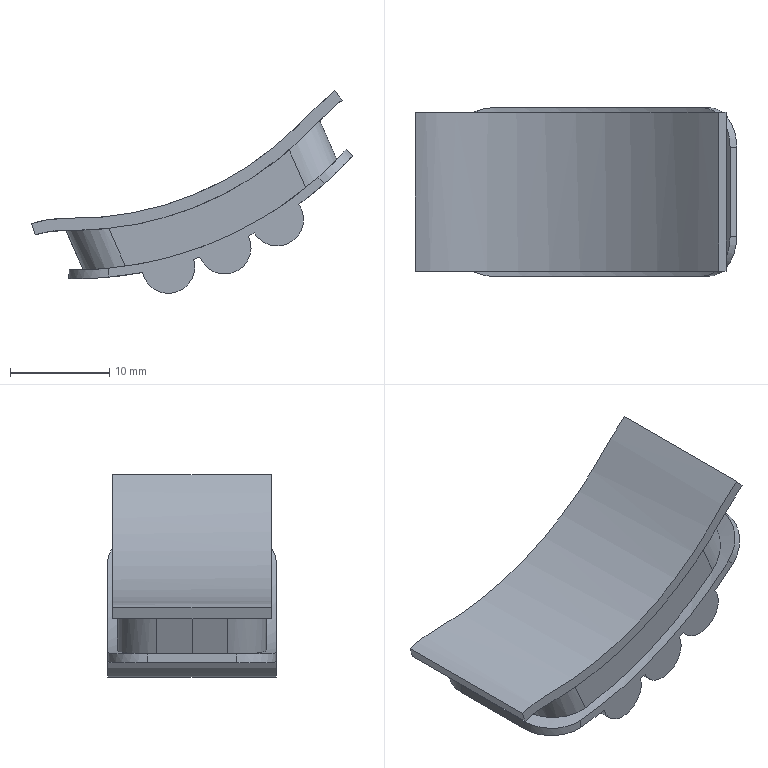Part | SolidWorks | features ICE 5, ExtruRefSurface 4, ExtendRefSurface 2, Fillet 2, Thicken 2, BossThin 1, CombineBodies 1, SewRefSurface 1, Shell 1, Stock 1, SurfCut 1, TrimRefSurface 1 | 1 solid | 31 faces | box 32.392 x 17 x 20.411 mm | volume 3378 mm3 | spline 11 | cylinder 11 | plane 9 | commonest cylinder face diameters 8 x8 5.337 x3